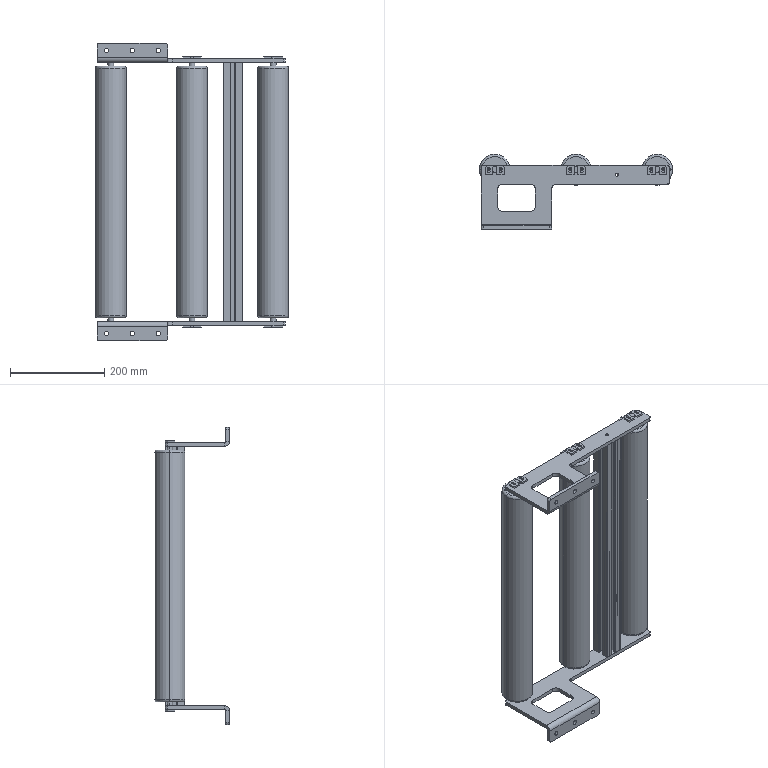Part | SolidWorks | features ReferencePattern 8, LocalLPattern 1, MirrorCompFeat 1 | 12 solids | 454 faces | box 410 x 159.5 x 631 mm | volume 6148104 mm3 | plane 298 | cylinder 140 | torus 12 | cone 4 | commonest cylinder face diameters 4 x26 4.2 x24 6 x24 9 x12 12 x12 20 x12